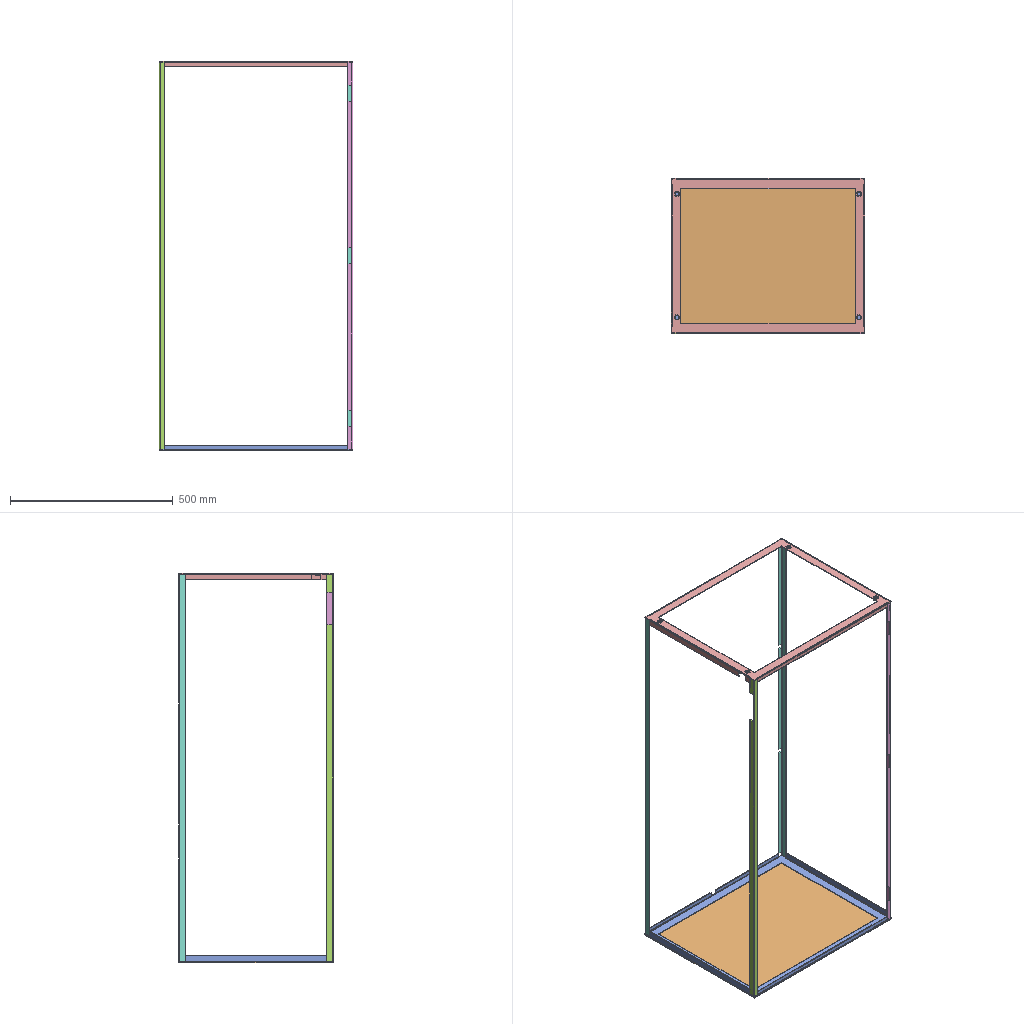Assembly | SolidWorks | 6 different items | 7 placed | box 596 x 476 x 1198 mm
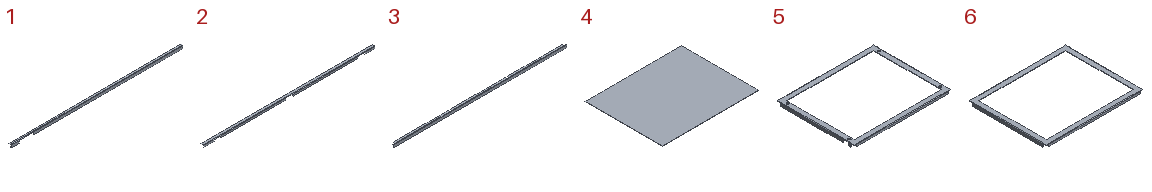Parts list (item | quantity | size | volume | features):
1 | x1 | 1191 x 15 x 20 mm | 90282 mm3 | features EdgeFlange 1, FlatPattern 1, ICE 1, SMBaseFlange 1, SheetMetal 1
2 | x1 | 1191 x 20 x 15 mm | 90032 mm3 | features LPattern 2, Cut 1, EdgeFlange 1, FlatPattern 1, ICE 1, SMBaseFlange 1, SheetMetal 1
3 | x2 | 1191 x 15 x 20 mm | 92732 mm3 | features EdgeFlange 1, FlatPattern 1, ICE 1, LPattern 1, MirrorPattern 1, SMBaseFlange 1, SheetMetal 1
4 | x1 | 596 x 476 x 1.5 mm | 425544 mm3 | features FlatPattern 1, SMBaseFlange 1, SheetMetal 1
5 | x1 | 596 x 476 x 20 mm | 219938 mm3 | features ICE 3, EdgeFlange 2, MirrorPattern 2, Cut 1, FlatPattern 1, LPattern 1, SMBaseFlange 1, SheetMetal 1
6 | x1 | 596 x 476 x 20 mm | 220905 mm3 | features EdgeFlange 2, MirrorPattern 2, FlatPattern 1, ICE 1, SMBaseFlange 1, SheetMetal 1
Mates (type | each side: item.copy, entity, surface, feature):
Coincident | 5.1 face plane Edge-Flange1 | 6.1 face plane Mirror2
Coincident | 5.1 face plane Edge-Flange2 | 6.1 face plane Edge-Flange2
DistanceDim | 6.1 face plane Base-Flange1 | 5.1 face plane Base-Flange1
Coincident | 5.1 face plane Edge-Flange2 | 1.1 face plane Base-Flange1
Coincident | 5.1 face plane Edge-Flange1 | 1.1 face plane Edge-Flange1
Coincident | 5.1 face plane Base-Flange1 | 1.1 face plane Base-Flange1
Coincident | 5.1 face plane Edge-Flange2 | 2.1 face plane Edge-Flange1
Coincident | 5.1 face plane Mirror2 | 2.1 face plane Base-Flange1
Coincident | 5.1 face plane Base-Flange1 | 2.1 face plane Edge-Flange1
Coincident | 5.1 face plane Edge-Flange1 | 3.1 face plane Edge-Flange1
Coincident | 5.1 face plane Mirror1 | 3.1 face plane Base-Flange1
Coincident | 5.1 face plane Mirror2 | 3.2 face plane Edge-Flange1
Coincident | 5.1 face plane Mirror1 | 3.2 face plane Base-Flange1
Coincident | 6.1 face plane Base-Flange1 | 3.1 face plane Edge-Flange1
Coincident | 6.1 face plane Base-Flange1 | 3.2 face plane Edge-Flange1
InPlace | 6.1 face plane Base-Flange1 | 4.1 plane